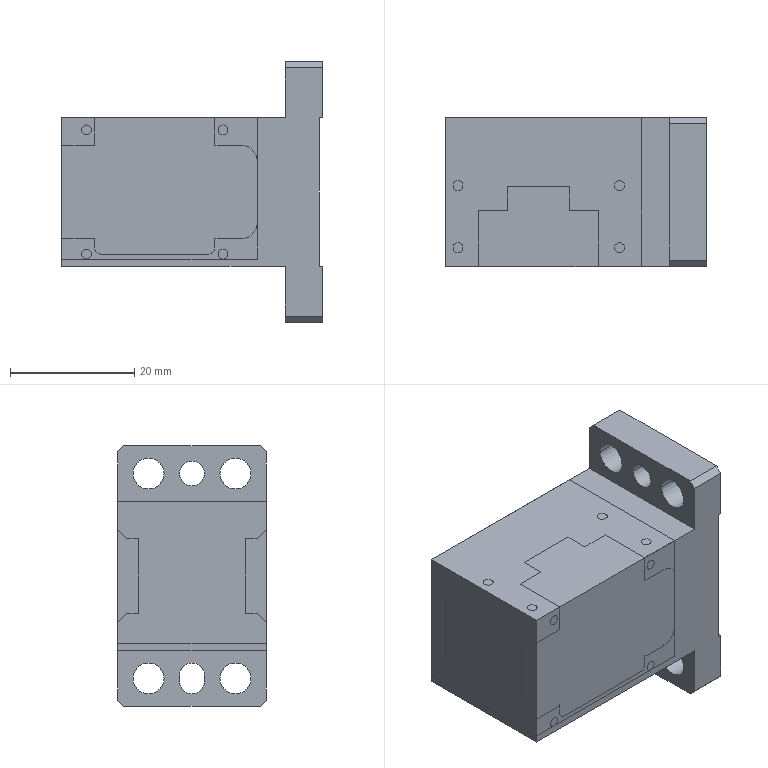NC program | NX | posted with a generic post | part box 42 x 24 x 42 mm
Lines 8757 to 8997 of 31406:
(FLOOR_WALL_1_1_COPY_1 , TOOL : D6JING)
N17512 T15 M6
N17514 G54
N17516 G17 G0 G90 X1. Y-14. B0. C0. S7500 M3
N17518 G43 Z30. H15
N17520 Z-1.93
N17522 G94 G1 Z-3.43 F1150.
N17524 X2.399 Y-16.52
N17526 G3 X2.699 Y-16. R0.6
N17528 G1 Y-24.
N17530 X-0.001
N17532 Y-16.
N17534 X-2.7
N17536 Y-24.
N17538 G3 X-2.4 Y-24.52 R0.6
N17540 G1 X0.164 Y-26.
N17542 Z-1.93
N17544 G0 Z30.
N17546 X0.136
N17548 Z-1.93
N17550 G1 Z-3.43
N17552 X2.7 Y-24.52
N17554 G3 X3. Y-24. R0.6
N17556 G1 Y-16.01
N17558 G3 X2.7 Y-15.49 R0.6
N17560 G1 X-2.7 Y-15.48
N17562 G3 X-3. Y-16. R0.6
N17564 G1 Y-24.
N17566 G3 X-2.7 Y-24.52 R0.6
N17568 G1 X-0.136 Y-26.
N17570 Z-1.93
N17572 G0 Z30.
N17574 X1. Y-12.1
N17576 Z-7.5
N17578 G1 Z-9.
N17580 X5.481
N17582 G3 X6.001 Y-12.4 R0.6
N17584 G1 Y-8.
N17586 X6.7
N17588 Y-12.4
N17590 Z-7.5
N17592 G0 Z30.
N17594 X1. Y-9.836
N17596 Z-7.5
N17598 G1 Z-9.
N17600 X2.48 Y-12.4
N17602 G3 X3. Y-12.7 R0.6
N17604 G1 X7.
N17606 Y-8.
N17608 G3 X6.7 Y-7.48 R0.6
N17610 G1 X4.136 Y-6.
N17612 Z-7.5
N17614 G0 Z30.
N17616 X1. Y-7.399
N17618 Z-11.34
N17620 G1 Z-12.84
N17622 X6.18
N17624 G3 X6.7 Y-7.699 R0.6
N17626 G1 X3.
N17628 Y-6.
N17630 X6.7
N17632 Y-4.3
N17634 X3.
N17636 G3 X2.48 Y-4.6 R0.6
N17638 G1 X1. Y-7.164
N17640 Z-11.34
N17642 G0 Z30.
N17644 Y-5.136
N17646 Z-11.34
N17648 G1 Z-12.84
N17650 X2.48 Y-7.7
N17652 G3 X3. Y-8. R0.6
N17654 G1 X7.
N17656 Y-4.
N17658 X3.
N17660 G3 X2.48 Y-4.3 R0.6
N17662 G1 X1. Y-6.864
N17664 Z-11.34
N17666 G0 Z30.
N17668 X3.137 Y-6.
N17670 Z-7.5
N17672 G1 Z-9.
N17674 X5.701 Y-4.52
N17676 G3 X6.001 Y-4. R0.6
N17678 G1 Y0.4
N17680 X6.7
N17682 Y-4.
N17684 G2 X6.4 Y-4.52 R0.6
N17686 G1 X3.836 Y-6.
N17688 Z-7.5
N17690 G0 Z30.
N17692 X4.136
N17694 Z-7.5
N17696 G1 Z-9.
N17698 X6.7 Y-4.52
N17700 G3 X7. Y-4. R0.6
N17702 G1 Y0.7
N17704 X3.
N17706 G3 X2.48 Y0.4 R0.6
N17708 G1 X1. Y-2.164
N17710 Z-7.5
N17712 G0 Z30.
N17714 Y2.
N17716 Z-1.93
N17718 G1 Z-3.43
N17720 X2.4 Y5.18
N17722 G3 X2.7 Y5.7 R0.6
N17724 G1 X-2.7
N17726 G3 X-2.4 Y5.18 R0.6
N17728 G1 X-1. Y2.
N17730 Z-1.93
N17732 G0 Z30.
N17734 X0.136
N17736 Z-1.93
N17738 G1 Z-3.43
N17740 X2.7 Y3.48
N17742 G3 X3. Y4. R0.6
N17744 G1 Y6.
N17746 X-3.
N17748 Y4.01
N17750 G3 X-2.7 Y3.49 R0.6
N17752 G1 X-0.119 Y2.
N17754 Z-1.93
N17756 G0 Z30.
N17758 X-1. Y-3.863
N17760 Z-7.5
N17762 G1 Z-9.
N17764 X-2.48 Y-1.299
N17766 G3 X-3. Y-0.999 R0.6
N17768 G1 X-15.
N17770 Y0.4
N17772 X-3.
N17774 G2 X-2.48 Y0.1 R0.6
N17776 G1 X-1. Y-2.464
N17778 Z-7.5
N17780 G0 Z30.
N17782 Y-2.164
N17784 Z-7.5
N17786 G1 Z-9.
N17788 X-2.48 Y0.4
N17790 G3 X-3. Y0.7 R0.6
N17792 G1 X-15.
N17794 G3 X-15.52 Y0.4 R0.6
N17796 G1 X-17. Y-2.164
N17798 Z-7.5
N17800 G0 Z30.
N17802 X-1. Y-7.399
N17804 Z-11.34
N17806 G1 Z-12.84
N17808 X-3.52
N17810 G3 X-3. Y-7.699 R0.6
N17812 G1 X-15.
N17814 Y-6.
N17816 X-3.
N17818 Y-4.3
N17820 X-15.
N17822 G3 X-15.52 Y-4.6 R0.6
N17824 G1 X-17. Y-7.164
N17826 Z-11.34
N17828 G0 Z30.
N17830 Y-5.136
N17832 Z-11.34
N17834 G1 Z-12.84
N17836 X-15.52 Y-7.7
N17838 G3 X-15. Y-8. R0.6
N17840 G1 X-3.
N17842 G3 X-2.48 Y-7.7 R0.6
N17844 G1 Y-4.3
N17846 G3 X-3. Y-4. R0.6
N17848 G1 X-15.
N17850 G3 X-15.52 Y-4.3 R0.6
N17852 G1 X-17. Y-6.864
N17854 Z-11.34
N17856 G0 Z30.
N17858 Y-8.137
N17860 Z-7.5
N17862 G1 Z-9.
N17864 X-15.52 Y-10.701
N17866 G3 X-15. Y-11.001 R0.6
N17868 G1 X-3.
N17870 Y-12.4
N17872 X-15.
N17874 G2 X-15.52 Y-12.1 R0.6
N17876 G1 X-17. Y-9.536
N17878 Z-7.5
N17880 G0 Z30.
N17882 Y-9.836
N17884 Z-7.5
N17886 G1 Z-9.
N17888 X-15.52 Y-12.4
N17890 G3 X-15. Y-12.7 R0.6
N17892 G1 X-3.
N17894 G3 X-2.48 Y-12.4 R0.6
N17896 G1 X-1. Y-9.836
N17898 Z-7.5
N17900 G0 Z30.
(CAVITY_MILL_COPY_1_COPY , TOOL : D6JING)
N17902 X1.73 Y-14.8
N17904 Z-7.
N17906 G1 Z-8. F1000.
N17908 X2.134 Y-15.5
N17910 G3 X3. Y-16. R1.
N17912 G1 Y4.
N17914 X-3.
N17916 Y-16.
N17918 X3.
N17920 G3 X2.5 Y-15.134 R1.
N17922 G1 X1.8 Y-14.73
N17924 Z-7.
N17926 G0 Z3.
N17928 X1.73 Y-14.8
N17930 Z-15.
N17932 G1 Z-16.
N17934 X2.134 Y-15.5
N17936 G3 X3. Y-16. R1.
N17938 G1 Y4.
N17940 X-3.
N17942 Y-16.
N17944 X3.
N17946 G3 X2.5 Y-15.134 R1.
N17948 G1 X1.8 Y-14.73
N17950 Z-15.
N17952 G0 Z-5.
N17954 X1.73 Y-14.8
N17956 Z-23.
N17958 G1 Z-24.
N17960 X2.134 Y-15.5
N17962 G3 X3. Y-16. R1.
N17964 G1 Y4.
N17966 X-3.
N17968 Y-16.
N17970 X3.
N17972 G3 X2.5 Y-15.134 R1.
N17974 G1 X1.8 Y-14.73
N17976 Z-23.
N17978 G0 Z30.
N17980 M5